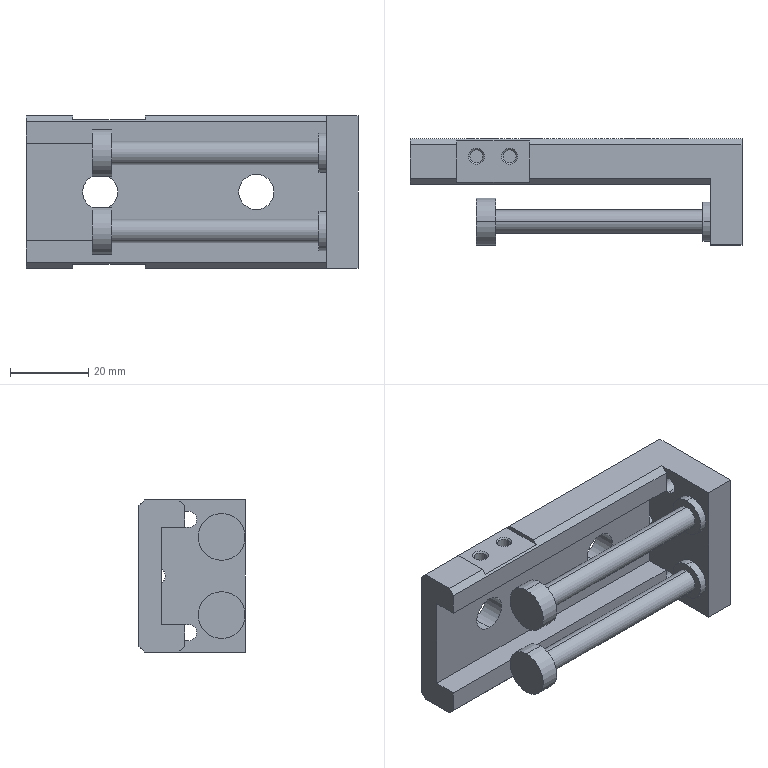Part | STEP file | 0246_Z_102_MXQ12L-30AS-A93_1 | 1 solid | 109 faces | box 85 x 27.2 x 39 mm | volume 34298 mm3 | plane 45 | cylinder 42 | cone 22 | commonest cylinder face diameters 3.3 x16 4.2 x6 4 x4 6 x4 9 x4 10 x4